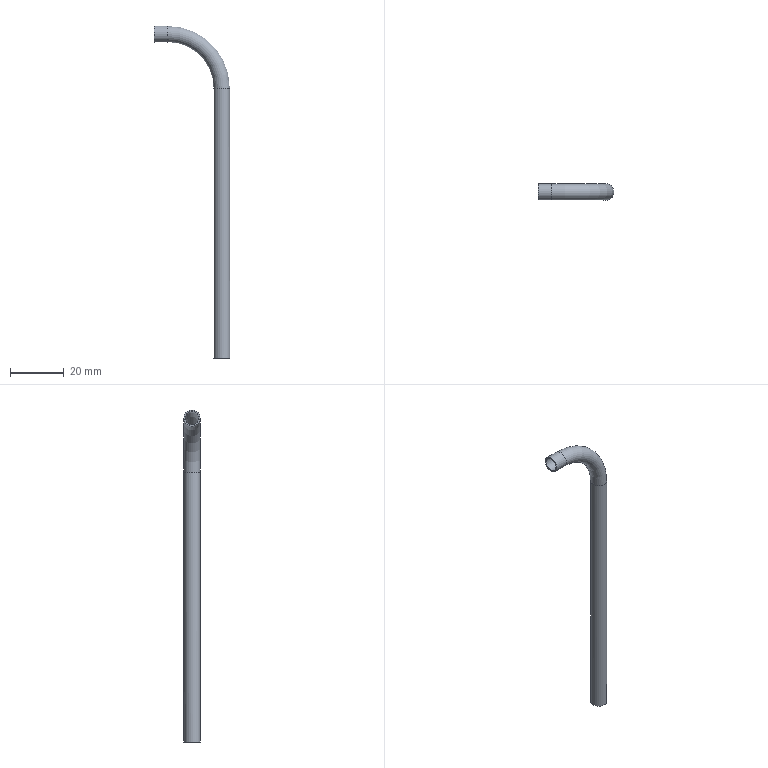Part | NX | features solid 2 | 1 solid | 8 faces | box 28 x 6 x 123 mm | volume 1179 mm3 | cylinder 4 | torus 2 | plane 2 | commonest cylinder face diameters 5 x2 6 x2
STEP:
#1=CARTESIAN_POINT('',(-280.,107.,120.));
#2=VERTEX_POINT('',#1);
#3=CARTESIAN_POINT('',(-280.,110.,120.));
#4=DIRECTION('',(0.,0.,1.));
#5=DIRECTION('',(0.,-1.,0.));
#6=AXIS2_PLACEMENT_3D('',#3,#4,#5);
#7=CIRCLE('',#6,3.);
#8=EDGE_CURVE('',#2,#2,#7,.T.);
#9=ORIENTED_EDGE('',*,*,#8,.F.);
#10=EDGE_LOOP('',(#9));
#11=FACE_BOUND('',#10,.T.);
#12=CARTESIAN_POINT('',(-277.,110.,20.));
#13=VERTEX_POINT('',#12);
#14=CARTESIAN_POINT('',(-280.,110.,20.));
#15=DIRECTION('',(0.,0.,1.));
#16=DIRECTION('',(1.,0.,0.));
#17=AXIS2_PLACEMENT_3D('',#14,#15,#16);
#18=CIRCLE('',#17,3.);
#19=EDGE_CURVE('',#13,#13,#18,.T.);
#20=ORIENTED_EDGE('',*,*,#19,.T.);
#21=EDGE_LOOP('',(#20));
#22=FACE_BOUND('',#21,.T.);
#23=CARTESIAN_POINT('',(-280.,110.,120.));
#24=DIRECTION('',(0.,0.,-1.));
#25=DIRECTION('',(0.,-1.,0.));
#26=AXIS2_PLACEMENT_3D('',#23,#24,#25);
#27=CYLINDRICAL_SURFACE('',#26,3.);
#28=ADVANCED_FACE('',(#11,#22),#27,.T.);
#29=CARTESIAN_POINT('',(-280.,107.5,120.));
#30=VERTEX_POINT('',#29);
#31=CARTESIAN_POINT('',(-280.,110.,120.));
#32=DIRECTION('',(0.,0.,1.));
#33=DIRECTION('',(0.,-1.,0.));
#34=AXIS2_PLACEMENT_3D('',#31,#32,#33);
#35=CIRCLE('',#34,2.5);
#36=EDGE_CURVE('',#30,#30,#35,.T.);
#37=ORIENTED_EDGE('',*,*,#36,.T.);
#38=EDGE_LOOP('',(#37));
#39=FACE_BOUND('',#38,.T.);
#40=CARTESIAN_POINT('',(-277.5,110.,20.));
#41=VERTEX_POINT('',#40);
#42=CARTESIAN_POINT('',(-280.,110.,20.));
#43=DIRECTION('',(0.,0.,1.));
#44=DIRECTION('',(1.,0.,0.));
#45=AXIS2_PLACEMENT_3D('',#42,#43,#44);
#46=CIRCLE('',#45,2.5);
#47=EDGE_CURVE('',#41,#41,#46,.T.);
#48=ORIENTED_EDGE('',*,*,#47,.F.);
#49=EDGE_LOOP('',(#48));
#50=FACE_BOUND('',#49,.T.);
#51=CARTESIAN_POINT('',(-280.,110.,120.));
#52=DIRECTION('',(0.,0.,-1.));
#53=DIRECTION('',(0.,-1.,0.));
#54=AXIS2_PLACEMENT_3D('',#51,#52,#53);
#55=CYLINDRICAL_SURFACE('',#54,2.5);
#56=ADVANCED_FACE('',(#39,#50),#55,.F.);
#57=CARTESIAN_POINT('',(-300.,107.,140.));
#58=VERTEX_POINT('',#57);
#59=CARTESIAN_POINT('',(-300.,110.,140.));
#60=DIRECTION('',(-1.,0.,0.));
#61=DIRECTION('',(0.,-1.,0.));
#62=AXIS2_PLACEMENT_3D('',#59,#60,#61);
#63=CIRCLE('',#62,3.);
#64=EDGE_CURVE('',#58,#58,#63,.T.);
#65=ORIENTED_EDGE('',*,*,#64,.F.);
#66=EDGE_LOOP('',(#65));
#67=FACE_BOUND('',#66,.T.);
#68=ORIENTED_EDGE('',*,*,#8,.T.);
#69=EDGE_LOOP('',(#68));
#70=FACE_BOUND('',#69,.T.);
#71=CARTESIAN_POINT('',(-300.,110.,120.));
#72=DIRECTION('',(0.,-1.,0.));
#73=DIRECTION('',(1.,0.,0.));
#74=AXIS2_PLACEMENT_3D('',#71,#72,#73);
#75=TOROIDAL_SURFACE('',#74,20.,3.);
#76=ADVANCED_FACE('',(#67,#70),#75,.T.);
#77=CARTESIAN_POINT('',(-300.,107.5,140.));
#78=VERTEX_POINT('',#77);
#79=CARTESIAN_POINT('',(-300.,110.,140.));
#80=DIRECTION('',(-1.,0.,0.));
#81=DIRECTION('',(0.,-1.,0.));
#82=AXIS2_PLACEMENT_3D('',#79,#80,#81);
#83=CIRCLE('',#82,2.5);
#84=EDGE_CURVE('',#78,#78,#83,.T.);
#85=ORIENTED_EDGE('',*,*,#84,.T.);
#86=EDGE_LOOP('',(#85));
#87=FACE_BOUND('',#86,.T.);
#88=ORIENTED_EDGE('',*,*,#36,.F.);
#89=EDGE_LOOP('',(#88));
#90=FACE_BOUND('',#89,.T.);
#91=CARTESIAN_POINT('',(-300.,110.,120.));
#92=DIRECTION('',(0.,-1.,0.));
#93=DIRECTION('',(1.,0.,0.));
#94=AXIS2_PLACEMENT_3D('',#91,#92,#93);
#95=TOROIDAL_SURFACE('',#94,20.,2.5);
#96=ADVANCED_FACE('',(#87,#90),#95,.F.);
#97=ORIENTED_EDGE('',*,*,#84,.F.);
#98=EDGE_LOOP('',(#97));
#99=FACE_BOUND('',#98,.T.);
#100=CARTESIAN_POINT('',(-305.,107.5,140.));
#101=VERTEX_POINT('',#100);
#102=CARTESIAN_POINT('',(-305.,110.,140.));
#103=DIRECTION('',(-1.,0.,0.));
#104=DIRECTION('',(0.,-1.,0.));
#105=AXIS2_PLACEMENT_3D('',#102,#103,#104);
#106=CIRCLE('',#105,2.5);
#107=EDGE_CURVE('',#101,#101,#106,.T.);
#108=ORIENTED_EDGE('',*,*,#107,.T.);
#109=EDGE_LOOP('',(#108));
#110=FACE_BOUND('',#109,.T.);
#111=CARTESIAN_POINT('',(-300.,110.,140.));
#112=DIRECTION('',(-1.,0.,0.));
#113=DIRECTION('',(0.,-1.,0.));
#114=AXIS2_PLACEMENT_3D('',#111,#112,#113);
#115=CYLINDRICAL_SURFACE('',#114,2.5);
#116=ADVANCED_FACE('',(#99,#110),#115,.F.);
#117=ORIENTED_EDGE('',*,*,#64,.T.);
#118=EDGE_LOOP('',(#117));
#119=FACE_BOUND('',#118,.T.);
#120=CARTESIAN_POINT('',(-305.,107.,140.));
#121=VERTEX_POINT('',#120);
#122=CARTESIAN_POINT('',(-305.,110.,140.));
#123=DIRECTION('',(-1.,0.,0.));
#124=DIRECTION('',(0.,-1.,0.));
#125=AXIS2_PLACEMENT_3D('',#122,#123,#124);
#126=CIRCLE('',#125,3.);
#127=EDGE_CURVE('',#121,#121,#126,.T.);
#128=ORIENTED_EDGE('',*,*,#127,.F.);
#129=EDGE_LOOP('',(#128));
#130=FACE_BOUND('',#129,.T.);
#131=CARTESIAN_POINT('',(-300.,110.,140.));
#132=DIRECTION('',(-1.,0.,0.));
#133=DIRECTION('',(0.,-1.,0.));
#134=AXIS2_PLACEMENT_3D('',#131,#132,#133);
#135=CYLINDRICAL_SURFACE('',#134,3.);
#136=ADVANCED_FACE('',(#119,#130),#135,.T.);
#137=ORIENTED_EDGE('',*,*,#47,.T.);
#138=EDGE_LOOP('',(#137));
#139=FACE_BOUND('',#138,.T.);
#140=ORIENTED_EDGE('',*,*,#19,.F.);
#141=EDGE_LOOP('',(#140));
#142=FACE_BOUND('',#141,.T.);
#143=CARTESIAN_POINT('',(-280.,110.,20.));
#144=DIRECTION('',(0.,0.,-1.));
#145=DIRECTION('',(0.,1.,0.));
#146=AXIS2_PLACEMENT_3D('',#143,#144,#145);
#147=PLANE('',#146);
#148=ADVANCED_FACE('',(#139,#142),#147,.T.);
#149=ORIENTED_EDGE('',*,*,#107,.F.);
#150=EDGE_LOOP('',(#149));
#151=FACE_BOUND('',#150,.T.);
#152=ORIENTED_EDGE('',*,*,#127,.T.);
#153=EDGE_LOOP('',(#152));
#154=FACE_BOUND('',#153,.T.);
#155=CARTESIAN_POINT('',(-305.,110.,140.));
#156=DIRECTION('',(1.,0.,0.));
#157=DIRECTION('',(0.,1.,0.));
#158=AXIS2_PLACEMENT_3D('',#155,#156,#157);
#159=PLANE('',#158);
#160=ADVANCED_FACE('',(#151,#154),#159,.F.);
#161=CLOSED_SHELL('',(#28,#56,#76,#96,#116,#136,#148,#160));
#162=MANIFOLD_SOLID_BREP('',#161);
#163=(LENGTH_UNIT()NAMED_UNIT(*)SI_UNIT(.MILLI.,.METRE.));
#164=UNCERTAINTY_MEASURE_WITH_UNIT(LENGTH_MEASURE(0.00001),#163,'','');
#165=(NAMED_UNIT(*)PLANE_ANGLE_UNIT()SI_UNIT($,.RADIAN.));
#166=(NAMED_UNIT(*)SI_UNIT($,.STERADIAN.)SOLID_ANGLE_UNIT());
#167=(GEOMETRIC_REPRESENTATION_CONTEXT(3)GLOBAL_UNCERTAINTY_ASSIGNED_CONTEXT((#164))GLOBAL_UNIT_ASSIGNED_CONTEXT((#163,#165,#166))REPRESENTATION_CONTEXT('',''));
#168=ADVANCED_BREP_SHAPE_REPRESENTATION('',(#162),#167);